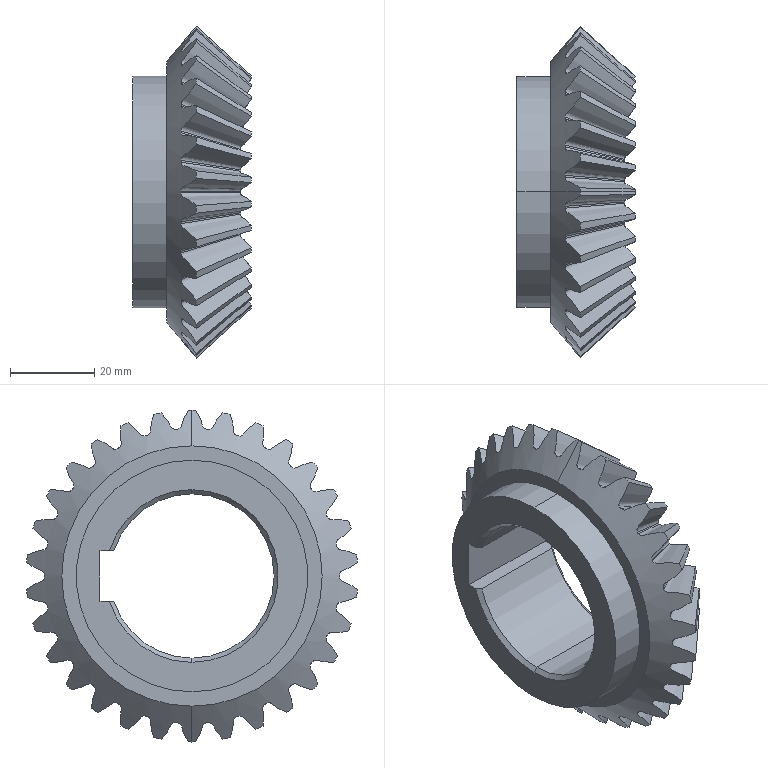Part | SolidWorks | features ICE 2, BlendCut 1, Chamfer 1, CirPattern 1, RefAxis 1, Revolution 1 | 1 solid | 171 faces | box 28.11 x 78.579 x 78.841 mm | volume 47773 mm3 | spline 90 | cone 70 | plane 6 | cylinder 5 | commonest cylinder face diameters 39 x3 55 x2